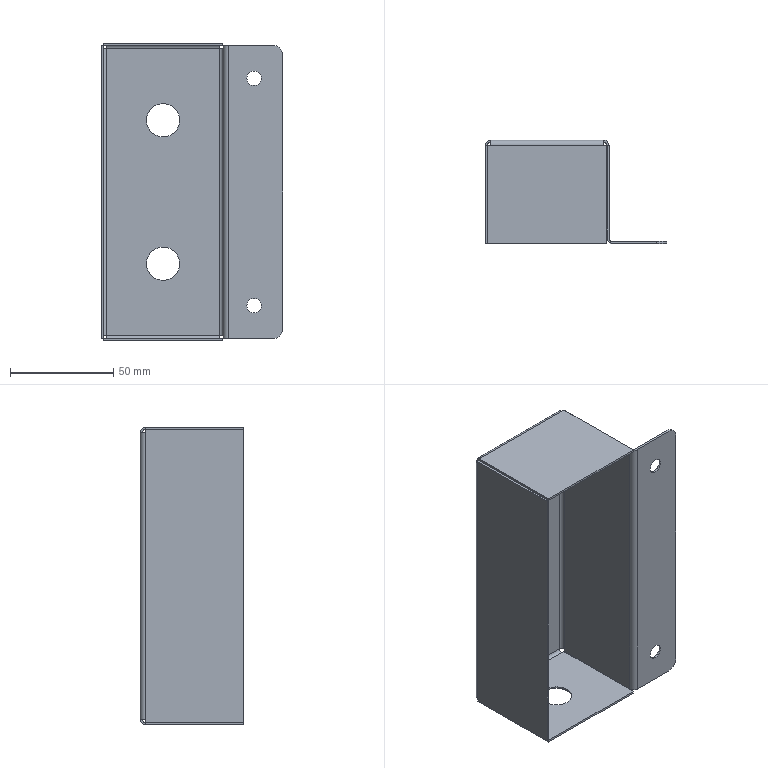Part | NX | 1 solid | 72 faces | box 88 x 50 x 144 mm | volume 30985 mm3 | plane 40 | cylinder 22 | cone 10 | commonest cylinder face diameters 3.2 x5 5.2 x5 7 x4 16.1 x4 10 x2 15 x2